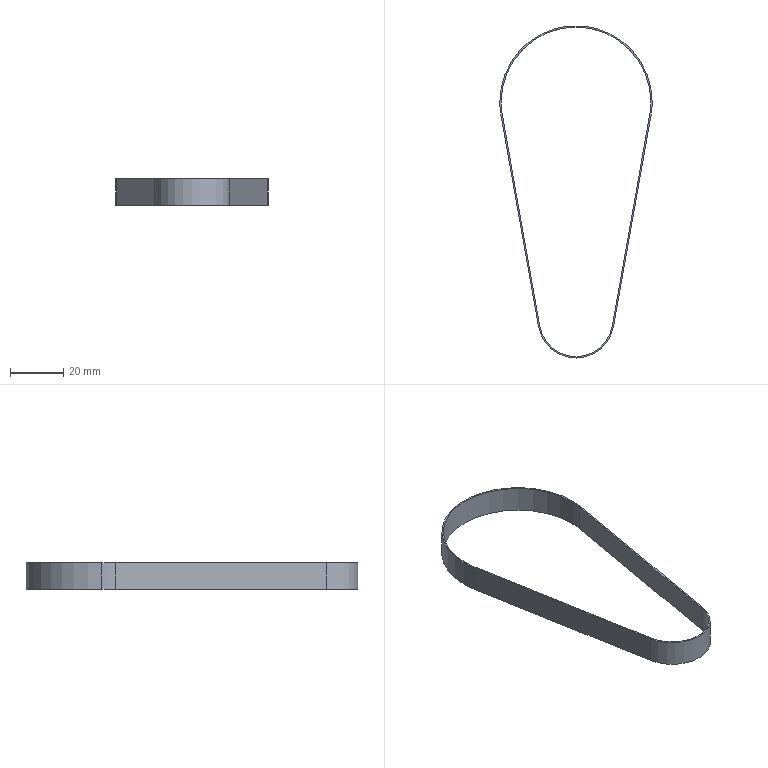Part | SolidWorks | features Extrusion 1 | 1 solid | 14 faces | box 57.3 x 124.975 x 10 mm | volume 1500 mm3 | cylinder 8 | plane 6 | commonest cylinder face diameters 56.3 x3 57.3 x3 27.65 x1 28.65 x1
STEP:
#1=CARTESIAN_POINT('',(27.717,77.082,5.));
#2=VERTEX_POINT('',#1);
#3=CARTESIAN_POINT('',(28.15,82.,5.));
#4=VERTEX_POINT('',#3);
#5=CARTESIAN_POINT('',(0.,82.,5.));
#6=DIRECTION('',(0.,0.,1.));
#7=DIRECTION('',(1.,0.,0.));
#8=AXIS2_PLACEMENT_3D('',#5,#6,#7);
#9=CIRCLE('',#8,28.15);
#10=EDGE_CURVE('',#2,#4,#9,.T.);
#11=ORIENTED_EDGE('',*,*,#10,.T.);
#12=CARTESIAN_POINT('',(28.15,82.,-5.));
#13=VERTEX_POINT('',#12);
#14=CARTESIAN_POINT('',(28.15,82.,5.));
#15=DIRECTION('',(0.,0.,-1.));
#16=VECTOR('',#15,1000.);
#17=LINE('',#14,#16);
#18=EDGE_CURVE('',#4,#13,#17,.T.);
#19=ORIENTED_EDGE('',*,*,#18,.T.);
#20=CARTESIAN_POINT('',(27.717,77.082,-5.));
#21=VERTEX_POINT('',#20);
#22=CARTESIAN_POINT('',(0.,82.,-5.));
#23=DIRECTION('',(0.,0.,1.));
#24=DIRECTION('',(1.,0.,0.));
#25=AXIS2_PLACEMENT_3D('',#22,#23,#24);
#26=CIRCLE('',#25,28.15);
#27=EDGE_CURVE('',#21,#13,#26,.T.);
#28=ORIENTED_EDGE('',*,*,#27,.F.);
#29=CARTESIAN_POINT('',(27.717,77.082,5.));
#30=DIRECTION('',(0.,0.,-1.));
#31=VECTOR('',#30,1000.);
#32=LINE('',#29,#31);
#33=EDGE_CURVE('',#2,#21,#32,.T.);
#34=ORIENTED_EDGE('',*,*,#33,.F.);
#35=EDGE_LOOP('',(#11,#19,#28,#34));
#36=FACE_OUTER_BOUND('',#35,.T.);
#37=CARTESIAN_POINT('',(0.,82.,5.));
#38=DIRECTION('',(0.,0.,-1.));
#39=DIRECTION('',(-1.,0.,0.));
#40=AXIS2_PLACEMENT_3D('',#37,#38,#39);
#41=CYLINDRICAL_SURFACE('',#40,28.15);
#42=ADVANCED_FACE('',(#36),#41,.F.);
#43=ORIENTED_EDGE('',*,*,#18,.F.);
#44=CARTESIAN_POINT('',(-28.15,82.,5.));
#45=VERTEX_POINT('',#44);
#46=CARTESIAN_POINT('',(0.,82.,5.));
#47=DIRECTION('',(0.,0.,1.));
#48=DIRECTION('',(1.,0.,0.));
#49=AXIS2_PLACEMENT_3D('',#46,#47,#48);
#50=CIRCLE('',#49,28.15);
#51=EDGE_CURVE('',#4,#45,#50,.T.);
#52=ORIENTED_EDGE('',*,*,#51,.T.);
#53=CARTESIAN_POINT('',(-28.15,82.,-5.));
#54=VERTEX_POINT('',#53);
#55=CARTESIAN_POINT('',(-28.15,82.,5.));
#56=DIRECTION('',(0.,0.,-1.));
#57=VECTOR('',#56,1000.);
#58=LINE('',#55,#57);
#59=EDGE_CURVE('',#45,#54,#58,.T.);
#60=ORIENTED_EDGE('',*,*,#59,.T.);
#61=CARTESIAN_POINT('',(0.,82.,-5.));
#62=DIRECTION('',(0.,0.,1.));
#63=DIRECTION('',(1.,0.,0.));
#64=AXIS2_PLACEMENT_3D('',#61,#62,#63);
#65=CIRCLE('',#64,28.15);
#66=EDGE_CURVE('',#13,#54,#65,.T.);
#67=ORIENTED_EDGE('',*,*,#66,.F.);
#68=EDGE_LOOP('',(#43,#52,#60,#67));
#69=FACE_OUTER_BOUND('',#68,.T.);
#70=CARTESIAN_POINT('',(0.,82.,5.));
#71=DIRECTION('',(0.,0.,-1.));
#72=DIRECTION('',(-1.,0.,0.));
#73=AXIS2_PLACEMENT_3D('',#70,#71,#72);
#74=CYLINDRICAL_SURFACE('',#73,28.15);
#75=ADVANCED_FACE('',(#69),#74,.F.);
#76=CARTESIAN_POINT('',(28.65,82.,5.));
#77=VERTEX_POINT('',#76);
#78=CARTESIAN_POINT('',(-28.65,82.,5.));
#79=VERTEX_POINT('',#78);
#80=CARTESIAN_POINT('',(0.,82.,5.));
#81=DIRECTION('',(0.,0.,1.));
#82=DIRECTION('',(1.,0.,0.));
#83=AXIS2_PLACEMENT_3D('',#80,#81,#82);
#84=CIRCLE('',#83,28.65);
#85=EDGE_CURVE('',#77,#79,#84,.T.);
#86=ORIENTED_EDGE('',*,*,#85,.F.);
#87=CARTESIAN_POINT('',(28.65,82.,-5.));
#88=VERTEX_POINT('',#87);
#89=CARTESIAN_POINT('',(28.65,82.,5.));
#90=DIRECTION('',(0.,0.,-1.));
#91=VECTOR('',#90,1000.);
#92=LINE('',#89,#91);
#93=EDGE_CURVE('',#77,#88,#92,.T.);
#94=ORIENTED_EDGE('',*,*,#93,.T.);
#95=CARTESIAN_POINT('',(-28.65,82.,-5.));
#96=VERTEX_POINT('',#95);
#97=CARTESIAN_POINT('',(0.,82.,-5.));
#98=DIRECTION('',(0.,0.,1.));
#99=DIRECTION('',(1.,0.,0.));
#100=AXIS2_PLACEMENT_3D('',#97,#98,#99);
#101=CIRCLE('',#100,28.65);
#102=EDGE_CURVE('',#88,#96,#101,.T.);
#103=ORIENTED_EDGE('',*,*,#102,.T.);
#104=CARTESIAN_POINT('',(-28.65,82.,5.));
#105=DIRECTION('',(0.,0.,-1.));
#106=VECTOR('',#105,1000.);
#107=LINE('',#104,#106);
#108=EDGE_CURVE('',#79,#96,#107,.T.);
#109=ORIENTED_EDGE('',*,*,#108,.F.);
#110=EDGE_LOOP('',(#86,#94,#103,#109));
#111=FACE_OUTER_BOUND('',#110,.T.);
#112=CARTESIAN_POINT('',(0.,82.,5.));
#113=DIRECTION('',(0.,0.,-1.));
#114=DIRECTION('',(-1.,0.,0.));
#115=AXIS2_PLACEMENT_3D('',#112,#113,#114);
#116=CYLINDRICAL_SURFACE('',#115,28.65);
#117=ADVANCED_FACE('',(#111),#116,.T.);
#118=CARTESIAN_POINT('',(-28.209,76.995,5.));
#119=VERTEX_POINT('',#118);
#120=CARTESIAN_POINT('',(0.,82.,5.));
#121=DIRECTION('',(0.,0.,1.));
#122=DIRECTION('',(1.,0.,0.));
#123=AXIS2_PLACEMENT_3D('',#120,#121,#122);
#124=CIRCLE('',#123,28.65);
#125=EDGE_CURVE('',#79,#119,#124,.T.);
#126=ORIENTED_EDGE('',*,*,#125,.F.);
#127=ORIENTED_EDGE('',*,*,#108,.T.);
#128=CARTESIAN_POINT('',(-28.209,76.995,-5.));
#129=VERTEX_POINT('',#128);
#130=CARTESIAN_POINT('',(0.,82.,-5.));
#131=DIRECTION('',(0.,0.,1.));
#132=DIRECTION('',(1.,0.,0.));
#133=AXIS2_PLACEMENT_3D('',#130,#131,#132);
#134=CIRCLE('',#133,28.65);
#135=EDGE_CURVE('',#96,#129,#134,.T.);
#136=ORIENTED_EDGE('',*,*,#135,.T.);
#137=CARTESIAN_POINT('',(-28.209,76.995,5.));
#138=DIRECTION('',(0.,0.,-1.));
#139=VECTOR('',#138,1000.);
#140=LINE('',#137,#139);
#141=EDGE_CURVE('',#119,#129,#140,.T.);
#142=ORIENTED_EDGE('',*,*,#141,.F.);
#143=EDGE_LOOP('',(#126,#127,#136,#142));
#144=FACE_OUTER_BOUND('',#143,.T.);
#145=CARTESIAN_POINT('',(0.,82.,5.));
#146=DIRECTION('',(0.,0.,-1.));
#147=DIRECTION('',(-1.,0.,0.));
#148=AXIS2_PLACEMENT_3D('',#145,#146,#147);
#149=CYLINDRICAL_SURFACE('',#148,28.65);
#150=ADVANCED_FACE('',(#144),#149,.T.);
#151=CARTESIAN_POINT('',(-14.105,-2.503,5.));
#152=VERTEX_POINT('',#151);
#153=CARTESIAN_POINT('',(14.105,-2.503,5.));
#154=VERTEX_POINT('',#153);
#155=CARTESIAN_POINT('',(0.,0.,5.));
#156=DIRECTION('',(0.,0.,1.));
#157=DIRECTION('',(1.,0.,0.));
#158=AXIS2_PLACEMENT_3D('',#155,#156,#157);
#159=CIRCLE('',#158,14.325);
#160=EDGE_CURVE('',#152,#154,#159,.T.);
#161=ORIENTED_EDGE('',*,*,#160,.T.);
#162=CARTESIAN_POINT('',(28.209,76.995,5.));
#163=VERTEX_POINT('',#162);
#164=CARTESIAN_POINT('',(28.209,76.995,5.));
#165=DIRECTION('',(0.1747,0.9846,0.));
#166=VECTOR('',#165,1000.);
#167=LINE('',#164,#166);
#168=EDGE_CURVE('',#154,#163,#167,.T.);
#169=ORIENTED_EDGE('',*,*,#168,.T.);
#170=CARTESIAN_POINT('',(0.,82.,5.));
#171=DIRECTION('',(0.,0.,1.));
#172=DIRECTION('',(1.,0.,0.));
#173=AXIS2_PLACEMENT_3D('',#170,#171,#172);
#174=CIRCLE('',#173,28.65);
#175=EDGE_CURVE('',#163,#77,#174,.T.);
#176=ORIENTED_EDGE('',*,*,#175,.T.);
#177=ORIENTED_EDGE('',*,*,#85,.T.);
#178=ORIENTED_EDGE('',*,*,#125,.T.);
#179=CARTESIAN_POINT('',(-28.209,76.995,5.));
#180=DIRECTION('',(0.1747,-0.9846,0.));
#181=VECTOR('',#180,1000.);
#182=LINE('',#179,#181);
#183=EDGE_CURVE('',#119,#152,#182,.T.);
#184=ORIENTED_EDGE('',*,*,#183,.T.);
#185=EDGE_LOOP('',(#161,#169,#176,#177,#178,#184));
#186=FACE_OUTER_BOUND('',#185,.T.);
#187=CARTESIAN_POINT('',(-27.717,77.082,5.));
#188=VERTEX_POINT('',#187);
#189=CARTESIAN_POINT('',(-13.612,-2.415,5.));
#190=VERTEX_POINT('',#189);
#191=CARTESIAN_POINT('',(-27.717,77.082,5.));
#192=DIRECTION('',(0.1747,-0.9846,0.));
#193=VECTOR('',#192,1000.);
#194=LINE('',#191,#193);
#195=EDGE_CURVE('',#188,#190,#194,.T.);
#196=ORIENTED_EDGE('',*,*,#195,.F.);
#197=CARTESIAN_POINT('',(0.,82.,5.));
#198=DIRECTION('',(0.,0.,1.));
#199=DIRECTION('',(1.,0.,0.));
#200=AXIS2_PLACEMENT_3D('',#197,#198,#199);
#201=CIRCLE('',#200,28.15);
#202=EDGE_CURVE('',#45,#188,#201,.T.);
#203=ORIENTED_EDGE('',*,*,#202,.F.);
#204=ORIENTED_EDGE('',*,*,#51,.F.);
#205=ORIENTED_EDGE('',*,*,#10,.F.);
#206=CARTESIAN_POINT('',(13.612,-2.415,5.));
#207=VERTEX_POINT('',#206);
#208=CARTESIAN_POINT('',(27.717,77.082,5.));
#209=DIRECTION('',(0.1747,0.9846,0.));
#210=VECTOR('',#209,1000.);
#211=LINE('',#208,#210);
#212=EDGE_CURVE('',#207,#2,#211,.T.);
#213=ORIENTED_EDGE('',*,*,#212,.F.);
#214=CARTESIAN_POINT('',(0.,0.,5.));
#215=DIRECTION('',(0.,0.,1.));
#216=DIRECTION('',(1.,0.,0.));
#217=AXIS2_PLACEMENT_3D('',#214,#215,#216);
#218=CIRCLE('',#217,13.825);
#219=EDGE_CURVE('',#190,#207,#218,.T.);
#220=ORIENTED_EDGE('',*,*,#219,.F.);
#221=EDGE_LOOP('',(#196,#203,#204,#205,#213,#220));
#222=FACE_BOUND('',#221,.T.);
#223=CARTESIAN_POINT('',(0.,0.,5.));
#224=DIRECTION('',(0.,0.,1.));
#225=DIRECTION('',(1.,0.,0.));
#226=AXIS2_PLACEMENT_3D('',#223,#224,#225);
#227=PLANE('',#226);
#228=ADVANCED_FACE('',(#186,#222),#227,.T.);
#229=CARTESIAN_POINT('',(-14.105,-2.503,-5.));
#230=VERTEX_POINT('',#229);
#231=CARTESIAN_POINT('',(14.105,-2.503,-5.));
#232=VERTEX_POINT('',#231);
#233=CARTESIAN_POINT('',(0.,0.,-5.));
#234=DIRECTION('',(0.,0.,1.));
#235=DIRECTION('',(1.,0.,0.));
#236=AXIS2_PLACEMENT_3D('',#233,#234,#235);
#237=CIRCLE('',#236,14.325);
#238=EDGE_CURVE('',#230,#232,#237,.T.);
#239=ORIENTED_EDGE('',*,*,#238,.F.);
#240=CARTESIAN_POINT('',(-28.209,76.995,-5.));
#241=DIRECTION('',(0.1747,-0.9846,0.));
#242=VECTOR('',#241,1000.);
#243=LINE('',#240,#242);
#244=EDGE_CURVE('',#129,#230,#243,.T.);
#245=ORIENTED_EDGE('',*,*,#244,.F.);
#246=ORIENTED_EDGE('',*,*,#135,.F.);
#247=ORIENTED_EDGE('',*,*,#102,.F.);
#248=CARTESIAN_POINT('',(28.209,76.995,-5.));
#249=VERTEX_POINT('',#248);
#250=CARTESIAN_POINT('',(0.,82.,-5.));
#251=DIRECTION('',(0.,0.,1.));
#252=DIRECTION('',(1.,0.,0.));
#253=AXIS2_PLACEMENT_3D('',#250,#251,#252);
#254=CIRCLE('',#253,28.65);
#255=EDGE_CURVE('',#249,#88,#254,.T.);
#256=ORIENTED_EDGE('',*,*,#255,.F.);
#257=CARTESIAN_POINT('',(28.209,76.995,-5.));
#258=DIRECTION('',(0.1747,0.9846,0.));
#259=VECTOR('',#258,1000.);
#260=LINE('',#257,#259);
#261=EDGE_CURVE('',#232,#249,#260,.T.);
#262=ORIENTED_EDGE('',*,*,#261,.F.);
#263=EDGE_LOOP('',(#239,#245,#246,#247,#256,#262));
#264=FACE_OUTER_BOUND('',#263,.T.);
#265=ORIENTED_EDGE('',*,*,#27,.T.);
#266=ORIENTED_EDGE('',*,*,#66,.T.);
#267=CARTESIAN_POINT('',(-27.717,77.082,-5.));
#268=VERTEX_POINT('',#267);
#269=CARTESIAN_POINT('',(0.,82.,-5.));
#270=DIRECTION('',(0.,0.,1.));
#271=DIRECTION('',(1.,0.,0.));
#272=AXIS2_PLACEMENT_3D('',#269,#270,#271);
#273=CIRCLE('',#272,28.15);
#274=EDGE_CURVE('',#54,#268,#273,.T.);
#275=ORIENTED_EDGE('',*,*,#274,.T.);
#276=CARTESIAN_POINT('',(-13.612,-2.415,-5.));
#277=VERTEX_POINT('',#276);
#278=CARTESIAN_POINT('',(-27.717,77.082,-5.));
#279=DIRECTION('',(0.1747,-0.9846,0.));
#280=VECTOR('',#279,1000.);
#281=LINE('',#278,#280);
#282=EDGE_CURVE('',#268,#277,#281,.T.);
#283=ORIENTED_EDGE('',*,*,#282,.T.);
#284=CARTESIAN_POINT('',(13.612,-2.415,-5.));
#285=VERTEX_POINT('',#284);
#286=CARTESIAN_POINT('',(0.,0.,-5.));
#287=DIRECTION('',(0.,0.,1.));
#288=DIRECTION('',(1.,0.,0.));
#289=AXIS2_PLACEMENT_3D('',#286,#287,#288);
#290=CIRCLE('',#289,13.825);
#291=EDGE_CURVE('',#277,#285,#290,.T.);
#292=ORIENTED_EDGE('',*,*,#291,.T.);
#293=CARTESIAN_POINT('',(27.717,77.082,-5.));
#294=DIRECTION('',(0.1747,0.9846,0.));
#295=VECTOR('',#294,1000.);
#296=LINE('',#293,#295);
#297=EDGE_CURVE('',#285,#21,#296,.T.);
#298=ORIENTED_EDGE('',*,*,#297,.T.);
#299=EDGE_LOOP('',(#265,#266,#275,#283,#292,#298));
#300=FACE_BOUND('',#299,.T.);
#301=CARTESIAN_POINT('',(0.,0.,-5.));
#302=DIRECTION('',(0.,0.,1.));
#303=DIRECTION('',(1.,0.,0.));
#304=AXIS2_PLACEMENT_3D('',#301,#302,#303);
#305=PLANE('',#304);
#306=ADVANCED_FACE('',(#264,#300),#305,.F.);
#307=ORIENTED_EDGE('',*,*,#238,.T.);
#308=CARTESIAN_POINT('',(14.105,-2.503,5.));
#309=DIRECTION('',(0.,0.,-1.));
#310=VECTOR('',#309,1000.);
#311=LINE('',#308,#310);
#312=EDGE_CURVE('',#154,#232,#311,.T.);
#313=ORIENTED_EDGE('',*,*,#312,.F.);
#314=ORIENTED_EDGE('',*,*,#160,.F.);
#315=CARTESIAN_POINT('',(-14.105,-2.503,5.));
#316=DIRECTION('',(0.,0.,-1.));
#317=VECTOR('',#316,1000.);
#318=LINE('',#315,#317);
#319=EDGE_CURVE('',#152,#230,#318,.T.);
#320=ORIENTED_EDGE('',*,*,#319,.T.);
#321=EDGE_LOOP('',(#307,#313,#314,#320));
#322=FACE_OUTER_BOUND('',#321,.T.);
#323=CARTESIAN_POINT('',(0.,0.,5.));
#324=DIRECTION('',(0.,0.,-1.));
#325=DIRECTION('',(-1.,0.,0.));
#326=AXIS2_PLACEMENT_3D('',#323,#324,#325);
#327=CYLINDRICAL_SURFACE('',#326,14.325);
#328=ADVANCED_FACE('',(#322),#327,.T.);
#329=ORIENTED_EDGE('',*,*,#261,.T.);
#330=CARTESIAN_POINT('',(28.209,76.995,5.));
#331=DIRECTION('',(0.,0.,-1.));
#332=VECTOR('',#331,1000.);
#333=LINE('',#330,#332);
#334=EDGE_CURVE('',#163,#249,#333,.T.);
#335=ORIENTED_EDGE('',*,*,#334,.F.);
#336=ORIENTED_EDGE('',*,*,#168,.F.);
#337=ORIENTED_EDGE('',*,*,#312,.T.);
#338=EDGE_LOOP('',(#329,#335,#336,#337));
#339=FACE_OUTER_BOUND('',#338,.T.);
#340=CARTESIAN_POINT('',(28.209,76.995,5.));
#341=DIRECTION('',(-0.9846,0.1747,0.));
#342=DIRECTION('',(-0.1747,-0.9846,0.));
#343=AXIS2_PLACEMENT_3D('',#340,#341,#342);
#344=PLANE('',#343);
#345=ADVANCED_FACE('',(#339),#344,.F.);
#346=ORIENTED_EDGE('',*,*,#93,.F.);
#347=ORIENTED_EDGE('',*,*,#175,.F.);
#348=ORIENTED_EDGE('',*,*,#334,.T.);
#349=ORIENTED_EDGE('',*,*,#255,.T.);
#350=EDGE_LOOP('',(#346,#347,#348,#349));
#351=FACE_OUTER_BOUND('',#350,.T.);
#352=CARTESIAN_POINT('',(0.,82.,5.));
#353=DIRECTION('',(0.,0.,-1.));
#354=DIRECTION('',(-1.,0.,0.));
#355=AXIS2_PLACEMENT_3D('',#352,#353,#354);
#356=CYLINDRICAL_SURFACE('',#355,28.65);
#357=ADVANCED_FACE('',(#351),#356,.T.);
#358=ORIENTED_EDGE('',*,*,#244,.T.);
#359=ORIENTED_EDGE('',*,*,#319,.F.);
#360=ORIENTED_EDGE('',*,*,#183,.F.);
#361=ORIENTED_EDGE('',*,*,#141,.T.);
#362=EDGE_LOOP('',(#358,#359,#360,#361));
#363=FACE_OUTER_BOUND('',#362,.T.);
#364=CARTESIAN_POINT('',(-28.209,76.995,5.));
#365=DIRECTION('',(0.9846,0.1747,0.));
#366=DIRECTION('',(-0.1747,0.9846,0.));
#367=AXIS2_PLACEMENT_3D('',#364,#365,#366);
#368=PLANE('',#367);
#369=ADVANCED_FACE('',(#363),#368,.F.);
#370=ORIENTED_EDGE('',*,*,#59,.F.);
#371=ORIENTED_EDGE('',*,*,#202,.T.);
#372=CARTESIAN_POINT('',(-27.717,77.082,5.));
#373=DIRECTION('',(0.,0.,-1.));
#374=VECTOR('',#373,1000.);
#375=LINE('',#372,#374);
#376=EDGE_CURVE('',#188,#268,#375,.T.);
#377=ORIENTED_EDGE('',*,*,#376,.T.);
#378=ORIENTED_EDGE('',*,*,#274,.F.);
#379=EDGE_LOOP('',(#370,#371,#377,#378));
#380=FACE_OUTER_BOUND('',#379,.T.);
#381=CARTESIAN_POINT('',(0.,82.,5.));
#382=DIRECTION('',(0.,0.,-1.));
#383=DIRECTION('',(-1.,0.,0.));
#384=AXIS2_PLACEMENT_3D('',#381,#382,#383);
#385=CYLINDRICAL_SURFACE('',#384,28.15);
#386=ADVANCED_FACE('',(#380),#385,.F.);
#387=ORIENTED_EDGE('',*,*,#282,.F.);
#388=ORIENTED_EDGE('',*,*,#376,.F.);
#389=ORIENTED_EDGE('',*,*,#195,.T.);
#390=CARTESIAN_POINT('',(-13.612,-2.415,5.));
#391=DIRECTION('',(0.,0.,-1.));
#392=VECTOR('',#391,1000.);
#393=LINE('',#390,#392);
#394=EDGE_CURVE('',#190,#277,#393,.T.);
#395=ORIENTED_EDGE('',*,*,#394,.T.);
#396=EDGE_LOOP('',(#387,#388,#389,#395));
#397=FACE_OUTER_BOUND('',#396,.T.);
#398=CARTESIAN_POINT('',(-27.717,77.082,5.));
#399=DIRECTION('',(0.9846,0.1747,0.));
#400=DIRECTION('',(-0.1747,0.9846,0.));
#401=AXIS2_PLACEMENT_3D('',#398,#399,#400);
#402=PLANE('',#401);
#403=ADVANCED_FACE('',(#397),#402,.T.);
#404=ORIENTED_EDGE('',*,*,#291,.F.);
#405=ORIENTED_EDGE('',*,*,#394,.F.);
#406=ORIENTED_EDGE('',*,*,#219,.T.);
#407=CARTESIAN_POINT('',(13.612,-2.415,5.));
#408=DIRECTION('',(0.,0.,-1.));
#409=VECTOR('',#408,1000.);
#410=LINE('',#407,#409);
#411=EDGE_CURVE('',#207,#285,#410,.T.);
#412=ORIENTED_EDGE('',*,*,#411,.T.);
#413=EDGE_LOOP('',(#404,#405,#406,#412));
#414=FACE_OUTER_BOUND('',#413,.T.);
#415=CARTESIAN_POINT('',(0.,0.,5.));
#416=DIRECTION('',(0.,0.,-1.));
#417=DIRECTION('',(-1.,0.,0.));
#418=AXIS2_PLACEMENT_3D('',#415,#416,#417);
#419=CYLINDRICAL_SURFACE('',#418,13.825);
#420=ADVANCED_FACE('',(#414),#419,.F.);
#421=ORIENTED_EDGE('',*,*,#297,.F.);
#422=ORIENTED_EDGE('',*,*,#411,.F.);
#423=ORIENTED_EDGE('',*,*,#212,.T.);
#424=ORIENTED_EDGE('',*,*,#33,.T.);
#425=EDGE_LOOP('',(#421,#422,#423,#424));
#426=FACE_OUTER_BOUND('',#425,.T.);
#427=CARTESIAN_POINT('',(27.717,77.082,5.));
#428=DIRECTION('',(-0.9846,0.1747,0.));
#429=DIRECTION('',(-0.1747,-0.9846,0.));
#430=AXIS2_PLACEMENT_3D('',#427,#428,#429);
#431=PLANE('',#430);
#432=ADVANCED_FACE('',(#426),#431,.T.);
#433=CLOSED_SHELL('',(#42,#75,#117,#150,#228,#306,#328,#345,#357,#369,#386,#403,#420,#432));
#434=MANIFOLD_SOLID_BREP('',#433);
#435=CARTESIAN_POINT('',(0.,0.,0.));
#436=DIRECTION('',(0.,0.,1.));
#437=DIRECTION('',(1.,0.,0.));
#438=AXIS2_PLACEMENT_3D('',#435,#436,#437);
#439=(LENGTH_UNIT()NAMED_UNIT(*)SI_UNIT(.MILLI.,.METRE.));
#440=UNCERTAINTY_MEASURE_WITH_UNIT(LENGTH_MEASURE(0.00001),#439,'','');
#441=(NAMED_UNIT(*)PLANE_ANGLE_UNIT()SI_UNIT($,.RADIAN.));
#442=(NAMED_UNIT(*)SI_UNIT($,.STERADIAN.)SOLID_ANGLE_UNIT());
#443=(GEOMETRIC_REPRESENTATION_CONTEXT(3)GLOBAL_UNCERTAINTY_ASSIGNED_CONTEXT((#440))GLOBAL_UNIT_ASSIGNED_CONTEXT((#439,#441,#442))REPRESENTATION_CONTEXT('',''));
#444=ADVANCED_BREP_SHAPE_REPRESENTATION('',(#434,#438),#443);